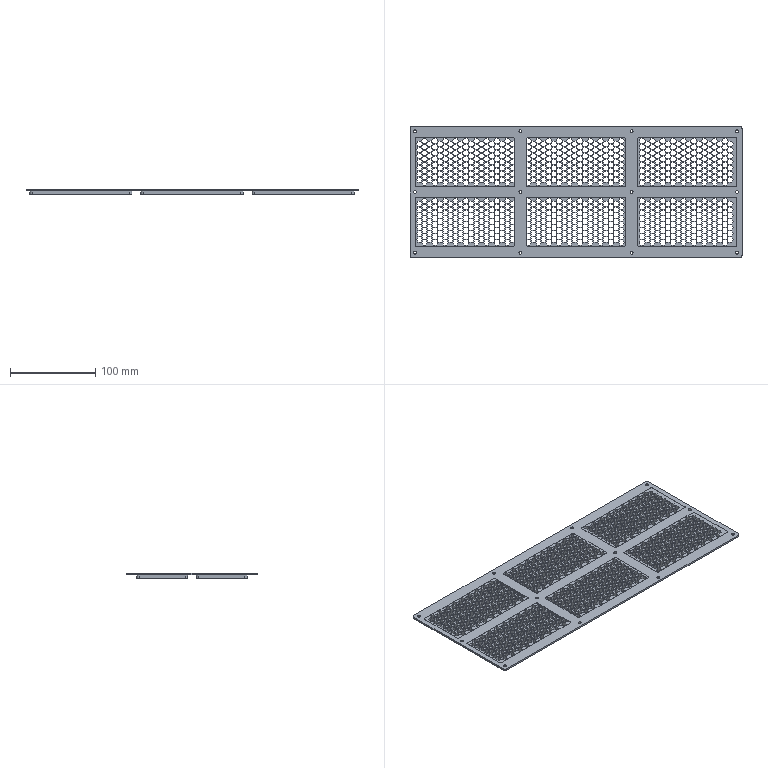NC program | NX | posted with a generic post
Lines 1 to 932 of 7861:
N10 G17 G21 G94 G90
(PLANAR_MILL , TOOL : D80R0.8)
N12 T01 M6
N14 G54
N16 G17 G0 G90 X251.5 Y-58.01 S3000 M3
N18 G43 Z50. H1
N20 Z2.
N22 G94 G1 Z0. F1000.
N24 X191.5
N26 X-191.5
N28 X-251.5
N30 Z2.
N32 G0 Z50.
N34 X251.5 Y-3.13
N36 Z2.
N38 G1 Z0.
N40 X191.5
N42 X-191.5
N44 X-251.5
N46 Z2.
N48 G0 Z50.
N50 X251.5 Y51.75
N52 Z2.
N54 G1 Z0.
N56 X191.5
N58 X-191.5
N60 X-251.5
N62 Z2.
N64 G0 Z50.
N66 M5
(PLANAR_MILL_1 , TOOL : D6_ROUGH)
N68 T02 M6
N70 G54
N72 G17 G0 G90 X156.765 Y-79.85 S5500 M3
N74 G43 Z50. H2
N76 Z1.
N78 G94 G1 X-192.093 Z0.817 F2000.
N80 X-193.653 Y-79.472 Z0.816
N82 X-195.052 Y-78.686
N84 X-196.186 Y-77.552 Z0.815
N86 X-196.972 Y-76.153 Z0.814
N88 X-197.35 Y-74.593 Z0.813
N90 Y74.593 Z0.735
N92 X-196.972 Y76.153 Z0.734
N94 X-196.186 Y77.552 Z0.733
N96 X-195.052 Y78.686
N98 X-193.653 Y79.472 Z0.732
N100 X-192.093 Y79.85 Z0.731
N102 X192.093 Z0.53
N104 X193.653 Y79.472 Z0.529
N106 X195.052 Y78.686 Z0.528
N108 X196.186 Y77.552 Z0.527
N110 X196.972 Y76.153 Z0.526
N112 X197.35 Y74.593 Z0.525
N114 Y-74.593 Z0.447
N116 X196.972 Y-76.153
N118 X196.186 Y-77.552 Z0.446
N120 X195.052 Y-78.686 Z0.445
N122 X193.653 Y-79.472 Z0.444
N124 X192.093 Y-79.85 Z0.443
N126 X-192.093 Z0.242
N128 X-193.653 Y-79.472 Z0.241
N130 X-195.052 Y-78.686 Z0.24
N132 X-196.186 Y-77.552 Z0.239
N134 X-196.972 Y-76.153
N136 X-197.35 Y-74.593 Z0.238
N138 Y74.593 Z0.16
N140 X-196.972 Y76.153 Z0.159
N142 X-196.186 Y77.552 Z0.158
N144 X-195.052 Y78.686 Z0.157
N146 X-193.653 Y79.472 Z0.156
N148 X-192.093 Y79.85 Z0.155
N150 X192.093 Z-0.046
N152 X193.653 Y79.472 Z-0.047
N154 X195.052 Y78.686
N156 X196.186 Y77.552 Z-0.048
N158 X196.972 Y76.153 Z-0.049
N160 X197.35 Y74.593 Z-0.05
N162 Y-74.593 Z-0.128
N164 X196.972 Y-76.153 Z-0.129
N166 X196.186 Y-77.552 Z-0.13
N168 X195.052 Y-78.686 Z-0.131
N170 X193.653 Y-79.472
N172 X192.093 Y-79.85 Z-0.132
N174 X-192.093 Z-0.333
N176 X-193.653 Y-79.472 Z-0.334
N178 X-195.052 Y-78.686 Z-0.335
N180 X-196.186 Y-77.552 Z-0.336
N182 X-196.972 Y-76.153 Z-0.337
N184 X-197.35 Y-74.593 Z-0.338
N186 Y74.593 Z-0.416
N188 X-196.972 Y76.153 Z-0.417
N190 X-196.186 Y77.552
N192 X-195.052 Y78.686 Z-0.418
N194 X-193.653 Y79.472 Z-0.419
N196 X-192.093 Y79.85 Z-0.42
N198 X192.093 Z-0.621
N200 X193.653 Y79.472 Z-0.622
N202 X195.052 Y78.686 Z-0.623
N204 X196.186 Y77.552 Z-0.624
N206 X196.972 Y76.153
N208 X197.35 Y74.593 Z-0.625
N210 Y-74.593 Z-0.703
N212 X196.972 Y-76.153 Z-0.704
N214 X196.186 Y-77.552 Z-0.705
N216 X195.052 Y-78.686 Z-0.706
N218 X193.653 Y-79.472 Z-0.707
N220 X192.093 Y-79.85 Z-0.708
N222 X-192.093 Z-0.909
N224 X-193.653 Y-79.472 Z-0.91
N226 X-195.052 Y-78.686
N228 X-196.186 Y-77.552 Z-0.911
N230 X-196.972 Y-76.153 Z-0.912
N232 X-197.35 Y-74.593 Z-0.913
N234 Y74.593 Z-0.991
N236 X-196.972 Y76.153 Z-0.992
N238 X-196.186 Y77.552 Z-0.993
N240 X-195.052 Y78.686 Z-0.994
N242 X-193.653 Y79.472
N244 X-192.093 Y79.85 Z-0.995
N246 X192.093 Z-1.196
N248 X193.653 Y79.472 Z-1.197
N250 X195.052 Y78.686 Z-1.198
N252 X196.186 Y77.552 Z-1.199
N254 X196.972 Y76.153 Z-1.2
N256 X197.35 Y74.593 Z-1.201
N258 Y-74.593 Z-1.279
N260 X196.972 Y-76.153 Z-1.28
N262 X196.186 Y-77.552
N264 X195.052 Y-78.686 Z-1.281
N266 X193.653 Y-79.472 Z-1.282
N268 X192.093 Y-79.85 Z-1.283
N270 X-192.093 Z-1.484
N272 X-193.653 Y-79.472 Z-1.485
N274 X-195.052 Y-78.686 Z-1.486
N276 X-196.186 Y-77.552 Z-1.487
N278 X-196.972 Y-76.153
N280 X-197.35 Y-74.593 Z-1.488
N282 Y74.593 Z-1.566
N284 X-196.972 Y76.153 Z-1.567
N286 X-196.186 Y77.552 Z-1.568
N288 X-195.052 Y78.686 Z-1.569
N290 X-193.653 Y79.472 Z-1.57
N292 X-192.093 Y79.85 Z-1.571
N294 X192.093 Z-1.772
N296 X193.653 Y79.472 Z-1.773
N298 X195.052 Y78.686
N300 X196.186 Y77.552 Z-1.774
N302 X196.972 Y76.153 Z-1.775
N304 X197.35 Y74.593 Z-1.776
N306 Y-74.593 Z-1.854
N308 X196.972 Y-76.153 Z-1.855
N310 X196.186 Y-77.552 Z-1.856
N312 X195.052 Y-78.686 Z-1.857
N314 X193.653 Y-79.472
N316 X192.093 Y-79.85 Z-1.858
N318 X-192.093 Z-2.059
N320 X-193.653 Y-79.472 Z-2.06
N322 X-195.052 Y-78.686 Z-2.061
N324 X-196.186 Y-77.552 Z-2.062
N326 X-196.972 Y-76.153 Z-2.063
N328 X-197.35 Y-74.593 Z-2.064
N330 Y74.593 Z-2.142
N332 X-196.972 Y76.153 Z-2.143
N334 X-196.186 Y77.552
N336 X-195.052 Y78.686 Z-2.144
N338 X-193.653 Y79.472 Z-2.145
N340 X-192.093 Y79.85 Z-2.146
N342 X192.093 Z-2.347
N344 X193.653 Y79.472 Z-2.348
N346 X195.052 Y78.686 Z-2.349
N348 X196.186 Y77.552 Z-2.35
N350 X196.972 Y76.153
N352 X197.35 Y74.593 Z-2.351
N354 Y-74.593 Z-2.429
N356 X196.972 Y-76.153 Z-2.43
N358 X196.186 Y-77.552 Z-2.431
N360 X195.052 Y-78.686 Z-2.432
N362 X193.653 Y-79.472 Z-2.433
N364 X192.093 Y-79.85 Z-2.434
N366 X-192.093 Z-2.635
N368 X-193.653 Y-79.472 Z-2.636
N370 X-195.052 Y-78.686
N372 X-196.186 Y-77.552 Z-2.637
N374 X-196.972 Y-76.153 Z-2.638
N376 X-197.35 Y-74.593 Z-2.639
N378 Y74.593 Z-2.717
N380 X-196.972 Y76.153 Z-2.718
N382 X-196.186 Y77.552 Z-2.719
N384 X-195.052 Y78.686 Z-2.72
N386 X-193.653 Y79.472
N388 X-192.093 Y79.85 Z-2.721
N390 X192.093 Z-2.922
N392 X193.653 Y79.472 Z-2.923
N394 X195.052 Y78.686 Z-2.924
N396 X196.186 Y77.552 Z-2.925
N398 X196.972 Y76.153 Z-2.926
N400 X197.35 Y74.593 Z-2.927
N402 Y-74.593 Z-3.005
N404 X196.972 Y-76.153 Z-3.006
N406 X196.186 Y-77.552
N408 X195.052 Y-78.686 Z-3.007
N410 X193.653 Y-79.472 Z-3.008
N412 X192.093 Y-79.85 Z-3.009
N414 X-192.093 Z-3.21
N416 X-193.653 Y-79.472 Z-3.211
N418 X-195.052 Y-78.686 Z-3.212
N420 X-196.186 Y-77.552 Z-3.213
N422 X-196.972 Y-76.153
N424 X-197.35 Y-74.593 Z-3.214
N426 Y74.593 Z-3.292
N428 X-196.972 Y76.153 Z-3.293
N430 X-196.186 Y77.552 Z-3.294
N432 X-195.052 Y78.686 Z-3.295
N434 X-193.653 Y79.472 Z-3.296
N436 X-192.093 Y79.85 Z-3.297
N438 X192.093 Z-3.498
N440 X193.653 Y79.472 Z-3.499
N442 X195.052 Y78.686
N444 X196.186 Y77.552 Z-3.5
N446 X196.972 Y76.153 Z-3.501
N448 X197.35 Y74.593 Z-3.502
N450 Y-74.593 Z-3.58
N452 X196.972 Y-76.153 Z-3.581
N454 X196.186 Y-77.552 Z-3.582
N456 X195.052 Y-78.686 Z-3.583
N458 X193.653 Y-79.472
N460 X192.093 Y-79.85 Z-3.584
N462 X-192.093 Z-3.785
N464 X-193.653 Y-79.472 Z-3.786
N466 X-195.052 Y-78.686 Z-3.787
N468 X-196.186 Y-77.552 Z-3.788
N470 X-196.972 Y-76.153 Z-3.789
N472 X-197.35 Y-74.593 Z-3.79
N474 Y74.593 Z-3.868
N476 X-196.972 Y76.153 Z-3.869
N478 X-196.186 Y77.552
N480 X-195.052 Y78.686 Z-3.87
N482 X-193.653 Y79.472 Z-3.871
N484 X-192.093 Y79.85 Z-3.872
N486 X192.093 Z-4.073
N488 X193.653 Y79.472 Z-4.074
N490 X195.052 Y78.686 Z-4.075
N492 X196.186 Y77.552 Z-4.076
N494 X196.972 Y76.153
N496 X197.35 Y74.593 Z-4.077
N498 Y-74.593 Z-4.155
N500 X196.972 Y-76.153 Z-4.156
N502 X196.186 Y-77.552 Z-4.157
N504 X195.052 Y-78.686 Z-4.158
N506 X193.653 Y-79.472 Z-4.159
N508 X192.093 Y-79.85 Z-4.16
N510 X-192.093 Z-4.361
N512 X-193.653 Y-79.472 Z-4.362
N514 X-195.052 Y-78.686
N516 X-196.186 Y-77.552 Z-4.363
N518 X-196.972 Y-76.153 Z-4.364
N520 X-197.35 Y-74.593 Z-4.365
N522 Y74.593 Z-4.443
N524 X-196.972 Y76.153 Z-4.444
N526 X-196.186 Y77.552 Z-4.445
N528 X-195.052 Y78.686 Z-4.446
N530 X-193.653 Y79.472
N532 X-192.093 Y79.85 Z-4.447
N534 X192.093 Z-4.648
N536 X193.653 Y79.472 Z-4.649
N538 X195.052 Y78.686 Z-4.65
N540 X196.186 Y77.552 Z-4.651
N542 X196.972 Y76.153 Z-4.652
N544 X197.35 Y74.593 Z-4.653
N546 Y-74.593 Z-4.731
N548 X196.972 Y-76.153 Z-4.732
N550 X196.186 Y-77.552
N552 X195.052 Y-78.686 Z-4.733
N554 X193.653 Y-79.472 Z-4.734
N556 X192.093 Y-79.85 Z-4.735
N558 X-192.093 Z-4.936
N560 X-193.653 Y-79.472 Z-4.937
N562 X-195.052 Y-78.686 Z-4.938
N564 X-196.186 Y-77.552 Z-4.939
N566 X-196.972 Y-76.153 Z-4.94
N568 X-197.35 Y-74.593
N570 Y74.593 Z-5.018
N572 X-196.972 Y76.153 Z-5.019
N574 X-196.186 Y77.552 Z-5.02
N576 X-195.052 Y78.686 Z-5.021
N578 X-193.653 Y79.472 Z-5.022
N580 X-192.093 Y79.85 Z-5.023
N582 X192.093 Z-5.224
N584 X193.653 Y79.472 Z-5.225
N586 X195.052 Y78.686 Z-5.226
N588 X196.186 Y77.552
N590 X196.972 Y76.153 Z-5.227
N592 X197.35 Y74.593 Z-5.228
N594 Y-74.593 Z-5.306
N596 X196.972 Y-76.153 Z-5.307
N598 X196.186 Y-77.552 Z-5.308
N600 X195.052 Y-78.686 Z-5.309
N602 X193.653 Y-79.472 Z-5.31
N604 X192.093 Y-79.85
N606 X-192.093 Z-5.512
N608 X-193.653 Y-79.472
N610 X-195.052 Y-78.686 Z-5.513
N612 X-196.186 Y-77.552 Z-5.514
N614 X-196.972 Y-76.153 Z-5.515
N616 X-197.35 Y-74.593 Z-5.516
N618 Y74.593 Z-5.594
N620 X-196.972 Y76.153 Z-5.595
N622 X-196.186 Y77.552 Z-5.596
N624 X-195.052 Y78.686
N626 X-193.653 Y79.472 Z-5.597
N628 X-192.093 Y79.85 Z-5.598
N630 X192.093 Z-5.799
N632 X193.653 Y79.472 Z-5.8
N634 X195.052 Y78.686 Z-5.801
N636 X196.186 Y77.552 Z-5.802
N638 X196.972 Y76.153 Z-5.803
N640 X197.35 Y74.593
N642 Y-74.593 Z-5.881
N644 X196.972 Y-76.153 Z-5.882
N646 X196.186 Y-77.552 Z-5.883
N648 X195.052 Y-78.686 Z-5.884
N650 X193.653 Y-79.472 Z-5.885
N652 X192.093 Y-79.85 Z-5.886
N654 X-192.093 Z-6.087
N656 X-193.653 Y-79.472 Z-6.088
N658 X-195.052 Y-78.686 Z-6.089
N660 X-196.186 Y-77.552
N662 X-196.972 Y-76.153 Z-6.09
N664 X-197.35 Y-74.593 Z-6.091
N666 Y74.593 Z-6.169
N668 X-196.972 Y76.153 Z-6.17
N670 X-196.186 Y77.552 Z-6.171
N672 X-195.052 Y78.686 Z-6.172
N674 X-193.653 Y79.472 Z-6.173
N676 X-192.093 Y79.85
N678 X192.093 Z-6.375
N680 X193.653 Y79.472
N682 X195.052 Y78.686 Z-6.376
N684 X196.186 Y77.552 Z-6.377
N686 X196.972 Y76.153 Z-6.378
N688 X197.35 Y74.593 Z-6.379
N690 Y-74.593 Z-6.457
N692 X196.972 Y-76.153 Z-6.458
N694 X196.186 Y-77.552 Z-6.459
N696 X195.052 Y-78.686
N698 X193.653 Y-79.472 Z-6.46
N700 X192.093 Y-79.85 Z-6.461
N702 X-192.093 Z-6.662
N704 X-193.653 Y-79.472 Z-6.663
N706 X-195.052 Y-78.686 Z-6.664
N708 X-196.186 Y-77.552 Z-6.665
N710 X-196.972 Y-76.153 Z-6.666
N712 X-197.35 Y-74.593
N714 Y74.593 Z-6.745
N716 X-196.972 Y76.153
N718 X-196.186 Y77.552 Z-6.746
N720 X-195.052 Y78.686 Z-6.747
N722 X-193.653 Y79.472 Z-6.748
N724 X-192.093 Y79.85 Z-6.749
N726 X192.093 Z-6.95
N728 X193.653 Y79.472 Z-6.951
N730 X195.052 Y78.686 Z-6.952
N732 X196.186 Y77.552
N734 X196.972 Y76.153 Z-6.953
N736 X197.35 Y74.593 Z-6.954
N738 Y-74.593 Z-7.032
N740 X196.972 Y-76.153 Z-7.033
N742 X196.186 Y-77.552 Z-7.034
N744 X195.052 Y-78.686 Z-7.035
N746 X193.653 Y-79.472 Z-7.036
N748 X192.093 Y-79.85
N750 X-192.093 Z-7.238
N752 X-193.653 Y-79.472
N754 X-195.052 Y-78.686 Z-7.239
N756 X-196.186 Y-77.552 Z-7.24
N758 X-196.972 Y-76.153 Z-7.241
N760 X-197.35 Y-74.593 Z-7.242
N762 Y74.593 Z-7.32
N764 X-196.972 Y76.153 Z-7.321
N766 X-196.186 Y77.552 Z-7.322
N768 X-195.052 Y78.686
N770 X-193.653 Y79.472 Z-7.323
N772 X-192.093 Y79.85 Z-7.324
N774 X192.093 Z-7.525
N776 X193.653 Y79.472 Z-7.526
N778 X195.052 Y78.686 Z-7.527
N780 X196.186 Y77.552 Z-7.528
N782 X196.972 Y76.153 Z-7.529
N784 X197.35 Y74.593
N786 Y-74.593 Z-7.608
N788 X196.972 Y-76.153
N790 X196.186 Y-77.552 Z-7.609
N792 X195.052 Y-78.686 Z-7.61
N794 X193.653 Y-79.472 Z-7.611
N796 X192.093 Y-79.85 Z-7.612
N798 X-192.093 Z-7.813
N800 X-193.653 Y-79.472 Z-7.814
N802 X-195.052 Y-78.686 Z-7.815
N804 X-196.186 Y-77.552
N806 X-196.972 Y-76.153 Z-7.816
N808 X-197.35 Y-74.593 Z-7.817
N810 Y74.593 Z-7.895
N812 X-196.972 Y76.153 Z-7.896
N814 X-196.186 Y77.552 Z-7.897
N816 X-195.052 Y78.686 Z-7.898
N818 X-193.653 Y79.472 Z-7.899
N820 X-192.093 Y79.85
N822 X0. Z-8.
N824 X191.5
N826 G2 X197.35 Y74. R5.85
N828 G1 Y-74.
N830 G2 X191.5 Y-79.85 R5.85
N832 G1 X-191.5
N834 G2 X-197.35 Y-74. R5.85
N836 G1 Y74.
N838 G2 X-191.5 Y79.85 R5.85
N840 G1 X0.
N842 Z-7.
N844 G0 Z50.
(PLANAR_MILL_1_COPY , TOOL : D6_ROUGH)
N846 X-191. Y-80.25 S4500
N848 Z-6.
N850 G1 Z-8. F800.
N852 G3 X-191.5 Y-79.75 R0.5
N854 G2 X-197.25 Y-74. R5.75
N856 G1 Y74.
N858 G2 X-191.5 Y79.75 R5.75
N860 G1 X191.5
N862 G2 X197.25 Y74. R5.75
N864 G1 Y-74.
N866 G2 X191.5 Y-79.75 R5.75
N868 G1 X-191.5
N870 G3 X-192. Y-80.25 R0.5
N872 G1 X-191.
N874 G3 X-191.5 Y-79.75 R0.5
N876 G2 X-197.25 Y-74. R5.75
N878 G1 Y74.
N880 G2 X-191.5 Y79.75 R5.75
N882 G1 X191.5
N884 G2 X197.25 Y74. R5.75
N886 G1 Y-74.
N888 G2 X191.5 Y-79.75 R5.75
N890 G1 X-191.5
N892 G3 X-192. Y-80.25 R0.5
N894 G1 Z-6.
N896 G0 Z50.
(FLOOR_FACING , TOOL : D6_ROUGH)
N898 Z52.9
N900 X-130.016 Y-29.65
N902 Z3.9
N904 G3 X-130.016 Y-29.65 Z3.011 I0.016 J-2.7
N906 X-130.016 Y-29.65 Z2.122 I0.016 J-2.7
N908 X-130.016 Y-29.65 Z1.233 I0.016 J-2.7
N910 X-130.016 Y-29.65 Z0.344 I0.016 J-2.7
N912 X-130. Y-35.05 Z-0.1 R2.7
N914 G1 X-99.95
N916 Y-34.95
N918 X-160.05
N920 Y-35.05
N922 X-130.
N924 Y-37.75
N926 X-97.25
N928 Y-32.25
N930 X-162.75
N932 Y-37.75
N934 X-130.
N936 Y-42.25
N938 X-92.75
N940 Y-27.75
N942 X-167.25
N944 Y-42.25
N946 X-130.
N948 Y-46.75
N950 X-88.25
N952 Y-23.25
N954 X-171.75
N956 Y-46.75
N958 X-130.
N960 Y-51.25
N962 X-83.75
N964 Y-18.75
N966 X-176.25
N968 Y-51.25
N970 X-130.
N972 Y-55.75
N974 X-79.25
N976 Y-14.25
N978 X-180.75
N980 Y-55.75
N982 X-130.
N984 Y-60.25
N986 X-74.75
N988 Y-9.75
N990 X-185.25
N992 Y-60.25
N994 X-130.
N996 X-129.
N998 Z0.9
N1000 G0 Z52.9
N1002 X-129.984 Y29.65
N1004 Z3.9
N1006 G3 X-129.984 Y29.65 Z3.011 I-0.016 J2.7
N1008 X-129.984 Y29.65 Z2.122 I-0.016 J2.7
N1010 X-129.984 Y29.65 Z1.233 I-0.016 J2.7
N1012 X-129.984 Y29.65 Z0.344 I-0.016 J2.7
N1014 X-130. Y35.05 Z-0.1 R2.7
N1016 G1 X-160.05
N1018 Y34.95
N1020 X-99.95
N1022 Y35.05
N1024 X-130.
N1026 Y37.75
N1028 X-162.75
N1030 Y32.25
N1032 X-97.25
N1034 Y37.75
N1036 X-130.
N1038 Y42.25
N1040 X-167.25
N1042 Y27.75
N1044 X-92.75
N1046 Y42.25
N1048 X-130.
N1050 Y46.75
N1052 X-171.75
N1054 Y23.25
N1056 X-88.25
N1058 Y46.75
N1060 X-130.
N1062 Y51.25
N1064 X-176.25
N1066 Y18.75
N1068 X-83.75
N1070 Y51.25
N1072 X-130.
N1074 Y55.75
N1076 X-180.75
N1078 Y14.25
N1080 X-79.25
N1082 Y55.75
N1084 X-130.
N1086 Y60.25
N1088 X-185.25
N1090 Y9.75
N1092 X-74.75
N1094 Y60.25
N1096 X-130.
N1098 X-131.
N1100 Z0.9
N1102 G0 Z52.9
N1104 X0.016 Y29.65
N1106 Z3.9
N1108 G3 X0.016 Y29.65 Z3.011 I-0.016 J2.7
N1110 X0.016 Y29.65 Z2.122 I-0.016 J2.7
N1112 X0.016 Y29.65 Z1.233 I-0.016 J2.7
N1114 X0.016 Y29.65 Z0.344 I-0.016 J2.7
N1116 X0. Y35.05 Z-0.1 R2.7
N1118 G1 X-30.05
N1120 Y34.95
N1122 X30.05
N1124 Y35.05
N1126 X0.
N1128 Y37.75
N1130 X-32.75
N1132 Y32.25
N1134 X32.75
N1136 Y37.75
N1138 X0.
N1140 Y42.25
N1142 X-37.25
N1144 Y27.75
N1146 X37.25
N1148 Y42.25
N1150 X0.
N1152 Y46.75
N1154 X-41.75
N1156 Y23.25
N1158 X41.75
N1160 Y46.75
N1162 X0.
N1164 Y51.25
N1166 X-46.25
N1168 Y18.75
N1170 X46.25
N1172 Y51.25
N1174 X0.
N1176 Y55.75
N1178 X-50.75
N1180 Y14.25
N1182 X50.75
N1184 Y55.75
N1186 X0.
N1188 Y60.25
N1190 X-55.25
N1192 Y9.75
N1194 X55.25
N1196 Y60.25
N1198 X0.
N1200 X-1.
N1202 Z0.9
N1204 G0 Z52.9
N1206 X-0.016 Y-29.65
N1208 Z3.9
N1210 G3 X-0.016 Y-29.65 Z3.011 I0.016 J-2.7
N1212 X-0.016 Y-29.65 Z2.122 I0.016 J-2.7
N1214 X-0.016 Y-29.65 Z1.233 I0.016 J-2.7
N1216 X-0.016 Y-29.65 Z0.344 I0.016 J-2.7
N1218 X0. Y-35.05 Z-0.1 R2.7
N1220 G1 X30.05
N1222 Y-34.95
N1224 X-30.05
N1226 Y-35.05
N1228 X0.
N1230 Y-37.75
N1232 X32.75
N1234 Y-32.25
N1236 X-32.75
N1238 Y-37.75
N1240 X0.
N1242 Y-42.25
N1244 X37.25
N1246 Y-27.75
N1248 X-37.25
N1250 Y-42.25
N1252 X0.
N1254 Y-46.75
N1256 X41.75
N1258 Y-23.25
N1260 X-41.75
N1262 Y-46.75
N1264 X0.
N1266 Y-51.25
N1268 X46.25
N1270 Y-18.75
N1272 X-46.25
N1274 Y-51.25
N1276 X0.
N1278 Y-55.75
N1280 X50.75
N1282 Y-14.25
N1284 X-50.75
N1286 Y-55.75
N1288 X0.
N1290 Y-60.25
N1292 X55.25
N1294 Y-9.75
N1296 X-55.25
N1298 Y-60.25
N1300 X0.
N1302 X1.
N1304 Z0.9
N1306 G0 Z52.9
N1308 X129.984 Y-29.65
N1310 Z3.9
N1312 G3 X129.984 Y-29.65 Z3.011 I0.016 J-2.7
N1314 X129.984 Y-29.65 Z2.122 I0.016 J-2.7
N1316 X129.984 Y-29.65 Z1.233 I0.016 J-2.7
N1318 X129.984 Y-29.65 Z0.344 I0.016 J-2.7
N1320 X130. Y-35.05 Z-0.1 R2.7
N1322 G1 X160.05
N1324 Y-34.95
N1326 X99.95
N1328 Y-35.05
N1330 X130.
N1332 Y-37.75
N1334 X162.75
N1336 Y-32.25
N1338 X97.25
N1340 Y-37.75
N1342 X130.
N1344 Y-42.25
N1346 X167.25
N1348 Y-27.75
N1350 X92.75
N1352 Y-42.25
N1354 X130.
N1356 Y-46.75
N1358 X171.75
N1360 Y-23.25
N1362 X88.25
N1364 Y-46.75
N1366 X130.
N1368 Y-51.25
N1370 X176.25
N1372 Y-18.75
N1374 X83.75
N1376 Y-51.25
N1378 X130.
N1380 Y-55.75
N1382 X180.75
N1384 Y-14.25
N1386 X79.25
N1388 Y-55.75
N1390 X130.
N1392 Y-60.25
N1394 X185.25
N1396 Y-9.75
N1398 X74.75
N1400 Y-60.25
N1402 X130.
N1404 X131.
N1406 Z0.9
N1408 G0 Z52.9
N1410 X130.016 Y29.65
N1412 Z3.9
N1414 G3 X130.016 Y29.65 Z3.011 I-0.016 J2.7
N1416 X130.016 Y29.65 Z2.122 I-0.016 J2.7
N1418 X130.016 Y29.65 Z1.233 I-0.016 J2.7
N1420 X130.016 Y29.65 Z0.344 I-0.016 J2.7
N1422 X130. Y35.05 Z-0.1 R2.7
N1424 G1 X99.95
N1426 Y34.95
N1428 X160.05
N1430 Y35.05
N1432 X130.
N1434 Y37.75
N1436 X97.25
N1438 Y32.25
N1440 X162.75
N1442 Y37.75
N1444 X130.
N1446 Y42.25
N1448 X92.75
N1450 Y27.75
N1452 X167.25
N1454 Y42.25
N1456 X130.
N1458 Y46.75
N1460 X88.25
N1462 Y23.25
N1464 X171.75
N1466 Y46.75
N1468 X130.
N1470 Y51.25
N1472 X83.75
N1474 Y18.75
N1476 X176.25
N1478 Y51.25
N1480 X130.
N1482 Y55.75
N1484 X79.25
N1486 Y14.25
N1488 X180.75
N1490 Y55.75
N1492 X130.
N1494 Y60.25
N1496 X74.75
N1498 Y9.75
N1500 X185.25
N1502 Y60.25
N1504 X130.
N1506 X129.
N1508 Z0.9
N1510 G0 Z52.9
N1512 M5
(PLANAR_MILL_2 , TOOL : D2_FINISH)
N1514 T03 M6
N1516 G54
N1518 G17 G0 G90 X-131. Y-61.25 S4500 M3
N1520 G43 Z50. H3
N1522 Z1.91
N1524 G94 G1 Z-0.09 F600.
N1526 G3 X-130. Y-62.25 R1.
N1528 G1 X-73.
N1530 G3 X-72.75 Y-62. R0.25
N1532 G1 Y-8.
N1534 G3 X-73. Y-7.75 R0.25
N1536 G1 X-187.
N1538 G3 X-187.25 Y-8. R0.25
N1540 G1 Y-62.
N1542 G3 X-187. Y-62.25 R0.25
N1544 G1 X-130.
N1546 G3 X-129. Y-61.25 R1.
N1548 G1 Z1.91
N1550 G0 Z50.
N1552 Y61.25
N1554 Z1.91
N1556 G1 Z-0.09
N1558 G3 X-130. Y62.25 R1.
N1560 G1 X-187.
N1562 G3 X-187.25 Y62. R0.25
N1564 G1 Y8.
N1566 G3 X-187. Y7.75 R0.25
N1568 G1 X-73.
N1570 G3 X-72.75 Y8. R0.25
N1572 G1 Y62.
N1574 G3 X-73. Y62.25 R0.25
N1576 G1 X-130.
N1578 G3 X-131. Y61.25 R1.
N1580 G1 Z1.91
N1582 G0 Z50.
N1584 X1.
N1586 Z1.91
N1588 G1 Z-0.09
N1590 G3 X0. Y62.25 R1.
N1592 G1 X-57.
N1594 G3 X-57.25 Y62. R0.25
N1596 G1 Y8.
N1598 G3 X-57. Y7.75 R0.25
N1600 G1 X57.
N1602 G3 X57.25 Y8. R0.25
N1604 G1 Y62.
N1606 G3 X57. Y62.25 R0.25
N1608 G1 X0.
N1610 G3 X-1. Y61.25 R1.
N1612 G1 Z1.91
N1614 G0 Z50.
N1616 Y-61.25
N1618 Z1.91
N1620 G1 Z-0.09
N1622 G3 X0. Y-62.25 R1.
N1624 G1 X57.
N1626 G3 X57.25 Y-62. R0.25
N1628 G1 Y-8.
N1630 G3 X57. Y-7.75 R0.25
N1632 G1 X-57.
N1634 G3 X-57.25 Y-8. R0.25
N1636 G1 Y-62.
N1638 G3 X-57. Y-62.25 R0.25
N1640 G1 X0.
N1642 G3 X1. Y-61.25 R1.
N1644 G1 Z1.91
N1646 G0 Z50.
N1648 X129.
N1650 Z1.91
N1652 G1 Z-0.09
N1654 G3 X130. Y-62.25 R1.
N1656 G1 X187.
N1658 G3 X187.25 Y-62. R0.25
N1660 G1 Y-8.
N1662 G3 X187. Y-7.75 R0.25
N1664 G1 X73.
N1666 G3 X72.75 Y-8. R0.25
N1668 G1 Y-62.
N1670 G3 X73. Y-62.25 R0.25
N1672 G1 X130.
N1674 G3 X131. Y-61.25 R1.
N1676 G1 Z1.91
N1678 G0 Z50.
N1680 Y61.25
N1682 Z1.91
N1684 G1 Z-0.09
N1686 G3 X130. Y62.25 R1.
N1688 G1 X73.
N1690 G3 X72.75 Y62. R0.25
N1692 G1 Y8.
N1694 G3 X73. Y7.75 R0.25
N1696 G1 X187.
N1698 G3 X187.25 Y8. R0.25
N1700 G1 Y62.
N1702 G3 X187. Y62.25 R0.25
N1704 G1 X130.
N1706 G3 X129. Y61.25 R1.
N1708 G1 Z1.91
N1710 G0 Z50.
N1712 M5
(PLANAR_MILL_1_COPY_COPY , TOOL : D4_CHAMFER)
N1714 T04 M6
N1716 G54
N1718 G17 G0 G90 X-189.5 Y-79.75 S3500 M3
N1720 G43 Z50. H4
N1722 Z1.
N1724 G94 G1 Z-1. F1000.
N1726 G3 X-191.5 Y-77.75 R2.
N1728 G2 X-195.25 Y-74. R3.75
N1730 G1 Y74.
N1732 G2 X-191.5 Y77.75 R3.75
N1734 G1 X191.5
N1736 G2 X195.25 Y74. R3.75
N1738 G1 Y-74.
N1740 G2 X191.5 Y-77.75 R3.75
N1742 G1 X-191.5
N1744 G3 X-193.5 Y-79.75 R2.
N1746 G1 Z1.
N1748 G0 Z50.
(DRILLING , TOOL : D4_CHAMFER)
N1750 X-188.5 Y71. S3000
N1752 Z30.
N1754 G81 G98 Z-1.75 F200. R3.
N1756 X-65.
N1758 X65.
N1760 X188.5
N1762 Y0.
N1764 X65.
N1766 X-65.
N1768 X-188.5
N1770 Y-71.
N1772 X-65.
N1774 X65.
N1776 X188.5
N1778 G80
N1780 G0 X188.5 Y-71. Z30.
N1782 M5
(DRILLING_COPY , TOOL : Z3.5)
N1784 T05 M6
N1786 G54
N1788 G17 G0 G90 X-188.5 Y71. S3000 M3
N1790 G43 Z30. H5
N1792 G94 G83 G98 Z-6. F200. Q2. R3.
N1794 X-65.
N1796 X65.
N1798 X188.5
N1800 Y0.
N1802 X65.
N1804 X-65.
N1806 X-188.5
N1808 Y-71.
N1810 X-65.
N1812 X65.
N1814 X188.5
N1816 G80
N1818 G0 X188.5 Y-71. Z30.
N1820 M5